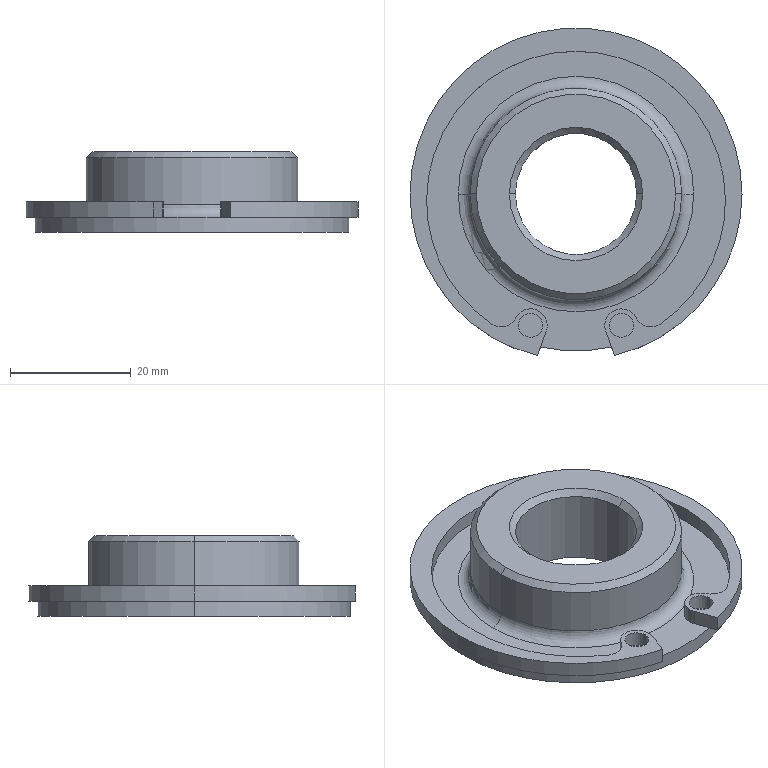Part | STEP file | CQ2A50-125DC-R06US_CQ2 SnapRing | 1 solid | 36 faces | box 55 x 54.243 x 13.3 mm | volume 12652 mm3 | cylinder 21 | plane 9 | cone 4 | torus 2 | commonest cylinder face diameters 5.5 x5 3.96 x4 49.5 x3 55 x3 20.1 x2 35 x2